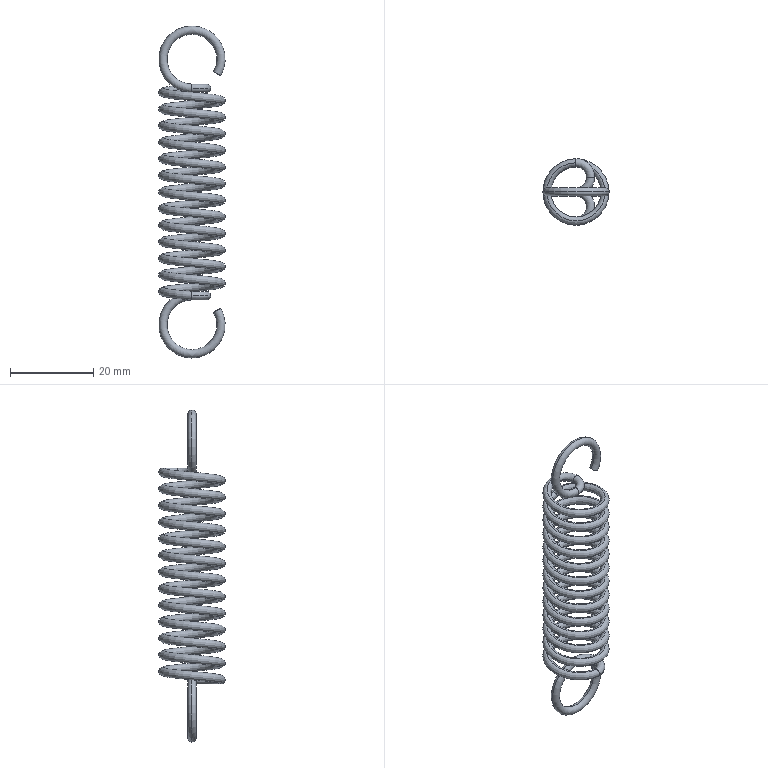Part | NX | features BREP 1 | 1 solid | 14 faces | box 16 x 16 x 80 mm | volume 1981 mm3 | torus 10 | plane 2 | spline 2